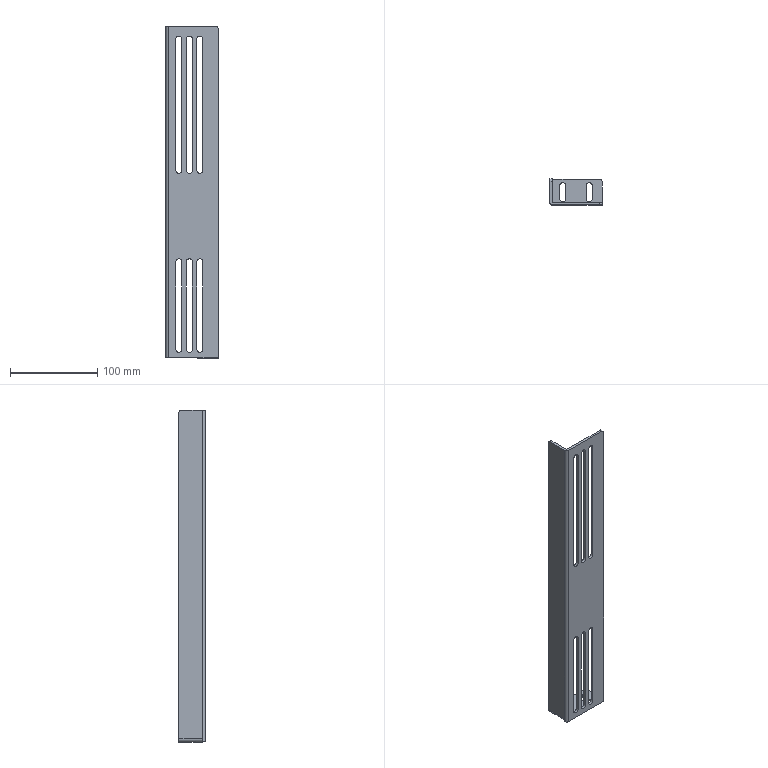Part | STEP file | X Travel Bracket | 1 solid | 58 faces | box 60 x 30 x 380 mm | volume 85607 mm3 | cylinder 29 | plane 29 | commonest cylinder face diameters 7 x23 6 x3 0.2 x1 1 x1 6.2 x1